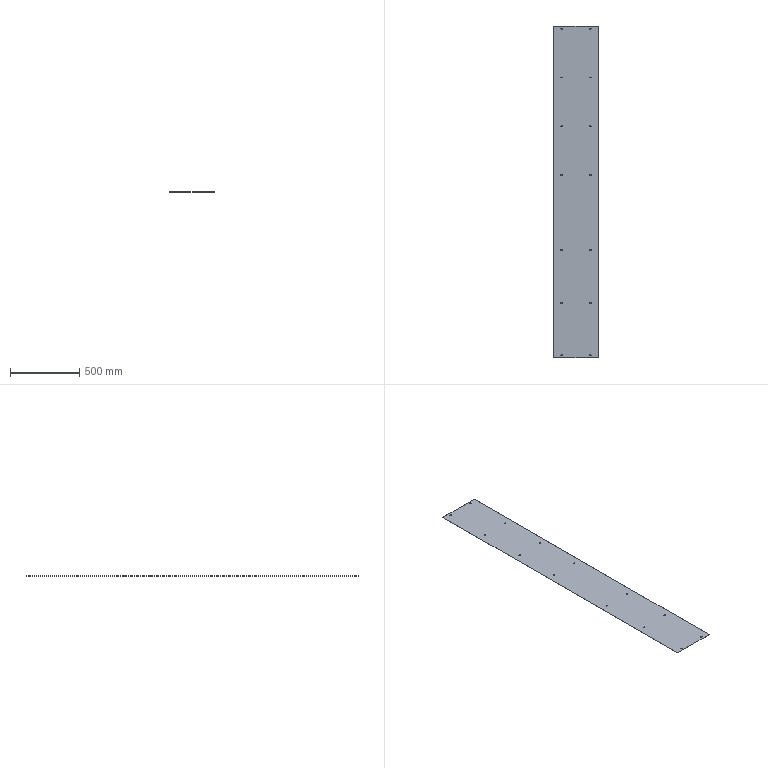Part | SolidWorks | features Extrusion 1, ICE 1 | 1 solid | 76 faces | box 322 x 2394 x 0.8 mm | volume 615975 mm3 | cylinder 42 | plane 34 | commonest cylinder face diameters 6 x42